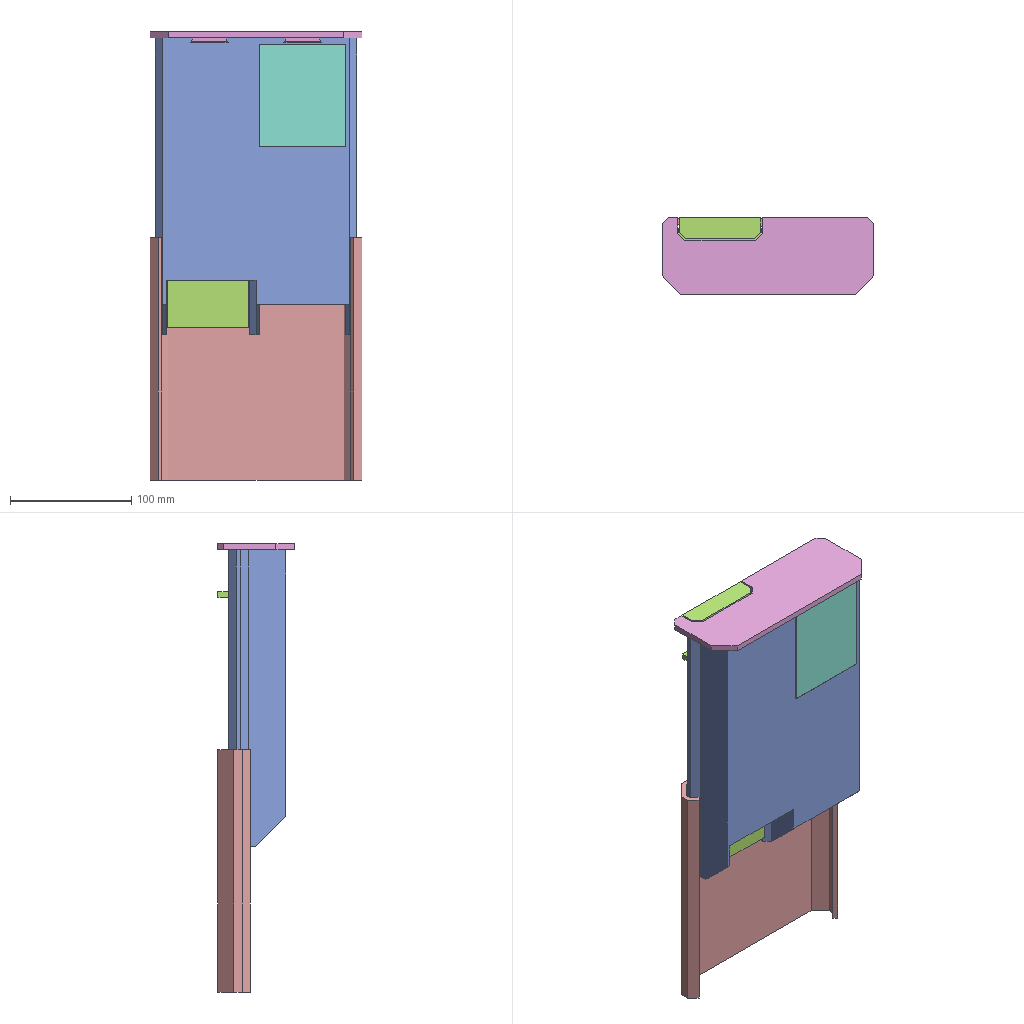Assembly | SolidWorks | 5 different items | 6 placed | box 175 x 63 x 370 mm
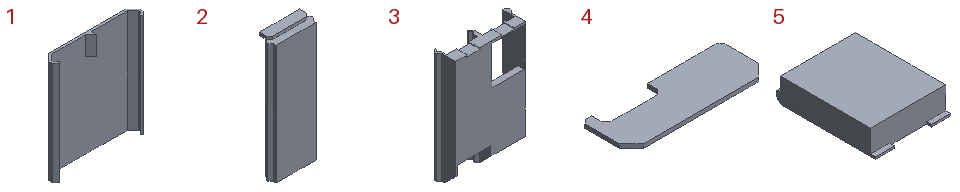Parts list (item | quantity | size | volume | features):
1 | x1 | 175 x 26.828 x 200 mm | 169317 mm3 | features ExtruThin 1, ICE 1
2 | x2 | 77 x 28 x 205 mm | 63647 mm3 | features Chamfer 1, Cut 1, Extrusion 1, ICE 1
3 | x1 | 166 x 47 x 245 mm | 294909 mm3 | features Cut 12, MoveFace 4, ICE 2, BossThin 1, Chamfer 1, CutThin 1, Extrusion 1
4 | x1 | 175 x 63 x 10 mm | 52854 mm3 | features Chamfer 2, ICE 2, Cut 1, Extrusion 1
5 | x1 | 70.6 x 92.5 x 23 mm | 56360 mm3 | features ICE 3, Cut 2, BossThin 1, DelFace 1, Extrusion 1, Fillet 1
Mates (type | each side: item.copy, entity, surface, feature):
InPlace | 1.1 plane | assembly plane
Coincident | 1.1 face plane Extrude-Thin1 | 3.1 face plane Boss-Extrude1 | 2 times
LimitDistanceDim | 1.1 face plane Extrude-Thin1 | 3.1 face plane Boss-Extrude1
InPlace | 3.1 face plane Boss-Extrude1 | 2.1 plane
Coincident | 3.1 face plane Cut-Extrude2 | 2.2 face plane Boss-Extrude1 | 2 times
LimitDistanceDim | 2.2 face plane Boss-Extrude1 | 1.1 face plane Extrude-Thin1
InPlace | 3.1 face plane Boss-Extrude1 | 4.1 plane
LimitDistanceDim | 2.2 face plane Boss-Extrude1 | 4.1 face plane Boss-Extrude1
InPlace | 3.1 face plane Cut-Extrude1 | assembly plane
InPlace | 3.1 face plane Boss-Extrude1 | 5.1 plane